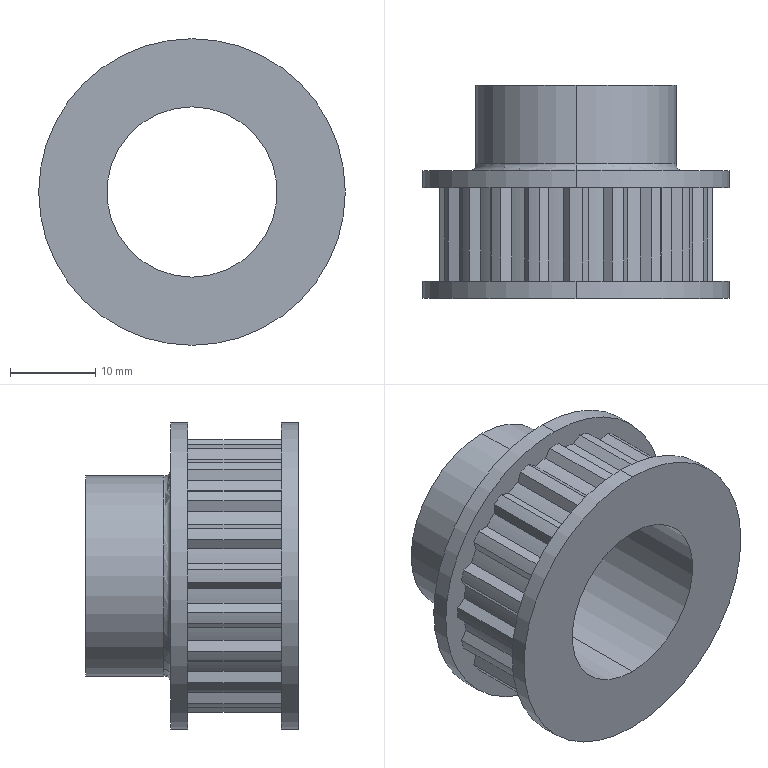Part | SolidWorks | features ICE 5, Extrusion 1, Fillet 1 | 1 solid | 96 faces | box 36 x 25 x 36 mm | volume 8830 mm3 | cylinder 49 | plane 45 | torus 2 | commonest cylinder face diameters 32 x21 30.016 x20 36 x4 20 x2 23.5 x2